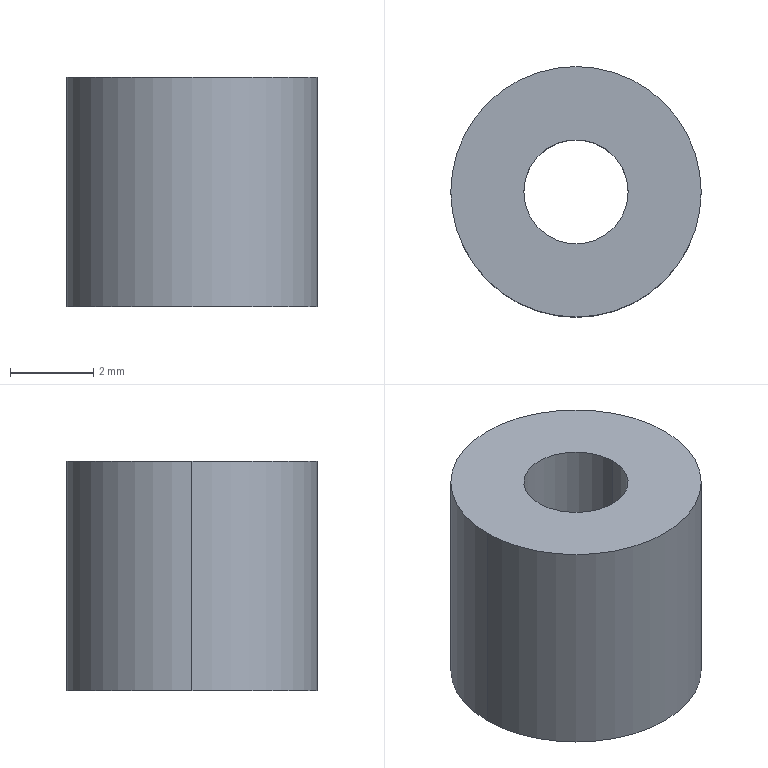Part | SolidWorks | features Extrusion 1 | 1 solid | 6 faces | box 6 x 6 x 5.5 mm | volume 128.511 mm3 | cylinder 4 | plane 2 | commonest cylinder face diameters 2.5 x2 6 x2
STEP:
#1=CARTESIAN_POINT('',(-1.25,0.,-2.75));
#2=VERTEX_POINT('',#1);
#3=CARTESIAN_POINT('',(1.25,0.,-2.75));
#4=VERTEX_POINT('',#3);
#5=CARTESIAN_POINT('',(0.,0.,-2.75));
#6=DIRECTION('',(0.,0.,1.));
#7=DIRECTION('',(1.,0.,0.));
#8=AXIS2_PLACEMENT_3D('',#5,#6,#7);
#9=CIRCLE('',#8,1.25);
#10=EDGE_CURVE('',#2,#4,#9,.T.);
#11=ORIENTED_EDGE('',*,*,#10,.F.);
#12=CARTESIAN_POINT('',(-1.25,0.,2.75));
#13=VERTEX_POINT('',#12);
#14=CARTESIAN_POINT('',(-1.25,0.,-2.75));
#15=DIRECTION('',(0.,0.,1.));
#16=VECTOR('',#15,1000.);
#17=LINE('',#14,#16);
#18=EDGE_CURVE('',#2,#13,#17,.T.);
#19=ORIENTED_EDGE('',*,*,#18,.T.);
#20=CARTESIAN_POINT('',(1.25,0.,2.75));
#21=VERTEX_POINT('',#20);
#22=CARTESIAN_POINT('',(0.,0.,2.75));
#23=DIRECTION('',(0.,0.,1.));
#24=DIRECTION('',(1.,0.,0.));
#25=AXIS2_PLACEMENT_3D('',#22,#23,#24);
#26=CIRCLE('',#25,1.25);
#27=EDGE_CURVE('',#13,#21,#26,.T.);
#28=ORIENTED_EDGE('',*,*,#27,.T.);
#29=CARTESIAN_POINT('',(1.25,0.,-2.75));
#30=DIRECTION('',(0.,0.,1.));
#31=VECTOR('',#30,1000.);
#32=LINE('',#29,#31);
#33=EDGE_CURVE('',#4,#21,#32,.T.);
#34=ORIENTED_EDGE('',*,*,#33,.F.);
#35=EDGE_LOOP('',(#11,#19,#28,#34));
#36=FACE_OUTER_BOUND('',#35,.T.);
#37=CARTESIAN_POINT('',(0.,0.,-2.75));
#38=DIRECTION('',(0.,0.,1.));
#39=DIRECTION('',(1.,0.,0.));
#40=AXIS2_PLACEMENT_3D('',#37,#38,#39);
#41=CYLINDRICAL_SURFACE('',#40,1.25);
#42=ADVANCED_FACE('',(#36),#41,.F.);
#43=CARTESIAN_POINT('',(3.,0.,-2.75));
#44=VERTEX_POINT('',#43);
#45=CARTESIAN_POINT('',(-3.,0.,-2.75));
#46=VERTEX_POINT('',#45);
#47=CARTESIAN_POINT('',(0.,0.,-2.75));
#48=DIRECTION('',(0.,0.,1.));
#49=DIRECTION('',(1.,0.,0.));
#50=AXIS2_PLACEMENT_3D('',#47,#48,#49);
#51=CIRCLE('',#50,3.);
#52=EDGE_CURVE('',#44,#46,#51,.T.);
#53=ORIENTED_EDGE('',*,*,#52,.T.);
#54=CARTESIAN_POINT('',(-3.,0.,2.75));
#55=VERTEX_POINT('',#54);
#56=CARTESIAN_POINT('',(-3.,0.,-2.75));
#57=DIRECTION('',(0.,0.,1.));
#58=VECTOR('',#57,1000.);
#59=LINE('',#56,#58);
#60=EDGE_CURVE('',#46,#55,#59,.T.);
#61=ORIENTED_EDGE('',*,*,#60,.T.);
#62=CARTESIAN_POINT('',(3.,0.,2.75));
#63=VERTEX_POINT('',#62);
#64=CARTESIAN_POINT('',(0.,0.,2.75));
#65=DIRECTION('',(0.,0.,1.));
#66=DIRECTION('',(1.,0.,0.));
#67=AXIS2_PLACEMENT_3D('',#64,#65,#66);
#68=CIRCLE('',#67,3.);
#69=EDGE_CURVE('',#63,#55,#68,.T.);
#70=ORIENTED_EDGE('',*,*,#69,.F.);
#71=CARTESIAN_POINT('',(3.,0.,-2.75));
#72=DIRECTION('',(0.,0.,1.));
#73=VECTOR('',#72,1000.);
#74=LINE('',#71,#73);
#75=EDGE_CURVE('',#44,#63,#74,.T.);
#76=ORIENTED_EDGE('',*,*,#75,.F.);
#77=EDGE_LOOP('',(#53,#61,#70,#76));
#78=FACE_OUTER_BOUND('',#77,.T.);
#79=CARTESIAN_POINT('',(0.,0.,-2.75));
#80=DIRECTION('',(0.,0.,1.));
#81=DIRECTION('',(1.,0.,0.));
#82=AXIS2_PLACEMENT_3D('',#79,#80,#81);
#83=CYLINDRICAL_SURFACE('',#82,3.);
#84=ADVANCED_FACE('',(#78),#83,.T.);
#85=ORIENTED_EDGE('',*,*,#60,.F.);
#86=CARTESIAN_POINT('',(0.,0.,-2.75));
#87=DIRECTION('',(0.,0.,1.));
#88=DIRECTION('',(1.,0.,0.));
#89=AXIS2_PLACEMENT_3D('',#86,#87,#88);
#90=CIRCLE('',#89,3.);
#91=EDGE_CURVE('',#46,#44,#90,.T.);
#92=ORIENTED_EDGE('',*,*,#91,.T.);
#93=ORIENTED_EDGE('',*,*,#75,.T.);
#94=CARTESIAN_POINT('',(0.,0.,2.75));
#95=DIRECTION('',(0.,0.,1.));
#96=DIRECTION('',(1.,0.,0.));
#97=AXIS2_PLACEMENT_3D('',#94,#95,#96);
#98=CIRCLE('',#97,3.);
#99=EDGE_CURVE('',#55,#63,#98,.T.);
#100=ORIENTED_EDGE('',*,*,#99,.F.);
#101=EDGE_LOOP('',(#85,#92,#93,#100));
#102=FACE_OUTER_BOUND('',#101,.T.);
#103=CARTESIAN_POINT('',(0.,0.,-2.75));
#104=DIRECTION('',(0.,0.,1.));
#105=DIRECTION('',(1.,0.,0.));
#106=AXIS2_PLACEMENT_3D('',#103,#104,#105);
#107=CYLINDRICAL_SURFACE('',#106,3.);
#108=ADVANCED_FACE('',(#102),#107,.T.);
#109=CARTESIAN_POINT('',(0.,0.,-2.75));
#110=DIRECTION('',(0.,0.,1.));
#111=DIRECTION('',(1.,0.,0.));
#112=AXIS2_PLACEMENT_3D('',#109,#110,#111);
#113=CIRCLE('',#112,1.25);
#114=EDGE_CURVE('',#4,#2,#113,.T.);
#115=ORIENTED_EDGE('',*,*,#114,.T.);
#116=ORIENTED_EDGE('',*,*,#10,.T.);
#117=EDGE_LOOP('',(#115,#116));
#118=FACE_BOUND('',#117,.T.);
#119=ORIENTED_EDGE('',*,*,#52,.F.);
#120=ORIENTED_EDGE('',*,*,#91,.F.);
#121=EDGE_LOOP('',(#119,#120));
#122=FACE_OUTER_BOUND('',#121,.T.);
#123=CARTESIAN_POINT('',(0.,0.,-2.75));
#124=DIRECTION('',(0.,0.,1.));
#125=DIRECTION('',(1.,0.,0.));
#126=AXIS2_PLACEMENT_3D('',#123,#124,#125);
#127=PLANE('',#126);
#128=ADVANCED_FACE('',(#118,#122),#127,.F.);
#129=CARTESIAN_POINT('',(0.,0.,2.75));
#130=DIRECTION('',(0.,0.,1.));
#131=DIRECTION('',(1.,0.,0.));
#132=AXIS2_PLACEMENT_3D('',#129,#130,#131);
#133=CIRCLE('',#132,1.25);
#134=EDGE_CURVE('',#21,#13,#133,.T.);
#135=ORIENTED_EDGE('',*,*,#134,.F.);
#136=ORIENTED_EDGE('',*,*,#27,.F.);
#137=EDGE_LOOP('',(#135,#136));
#138=FACE_BOUND('',#137,.T.);
#139=ORIENTED_EDGE('',*,*,#69,.T.);
#140=ORIENTED_EDGE('',*,*,#99,.T.);
#141=EDGE_LOOP('',(#139,#140));
#142=FACE_OUTER_BOUND('',#141,.T.);
#143=CARTESIAN_POINT('',(0.,0.,2.75));
#144=DIRECTION('',(0.,0.,1.));
#145=DIRECTION('',(1.,0.,0.));
#146=AXIS2_PLACEMENT_3D('',#143,#144,#145);
#147=PLANE('',#146);
#148=ADVANCED_FACE('',(#138,#142),#147,.T.);
#149=ORIENTED_EDGE('',*,*,#18,.F.);
#150=ORIENTED_EDGE('',*,*,#114,.F.);
#151=ORIENTED_EDGE('',*,*,#33,.T.);
#152=ORIENTED_EDGE('',*,*,#134,.T.);
#153=EDGE_LOOP('',(#149,#150,#151,#152));
#154=FACE_OUTER_BOUND('',#153,.T.);
#155=CARTESIAN_POINT('',(0.,0.,-2.75));
#156=DIRECTION('',(0.,0.,1.));
#157=DIRECTION('',(1.,0.,0.));
#158=AXIS2_PLACEMENT_3D('',#155,#156,#157);
#159=CYLINDRICAL_SURFACE('',#158,1.25);
#160=ADVANCED_FACE('',(#154),#159,.F.);
#161=CLOSED_SHELL('',(#42,#84,#108,#128,#148,#160));
#162=MANIFOLD_SOLID_BREP('',#161);
#163=CARTESIAN_POINT('',(0.,0.,0.));
#164=DIRECTION('',(0.,0.,1.));
#165=DIRECTION('',(1.,0.,0.));
#166=AXIS2_PLACEMENT_3D('',#163,#164,#165);
#167=(LENGTH_UNIT()NAMED_UNIT(*)SI_UNIT(.MILLI.,.METRE.));
#168=UNCERTAINTY_MEASURE_WITH_UNIT(LENGTH_MEASURE(0.00001),#167,'','');
#169=(NAMED_UNIT(*)PLANE_ANGLE_UNIT()SI_UNIT($,.RADIAN.));
#170=(NAMED_UNIT(*)SI_UNIT($,.STERADIAN.)SOLID_ANGLE_UNIT());
#171=(GEOMETRIC_REPRESENTATION_CONTEXT(3)GLOBAL_UNCERTAINTY_ASSIGNED_CONTEXT((#168))GLOBAL_UNIT_ASSIGNED_CONTEXT((#167,#169,#170))REPRESENTATION_CONTEXT('',''));
#172=ADVANCED_BREP_SHAPE_REPRESENTATION('',(#162,#166),#171);